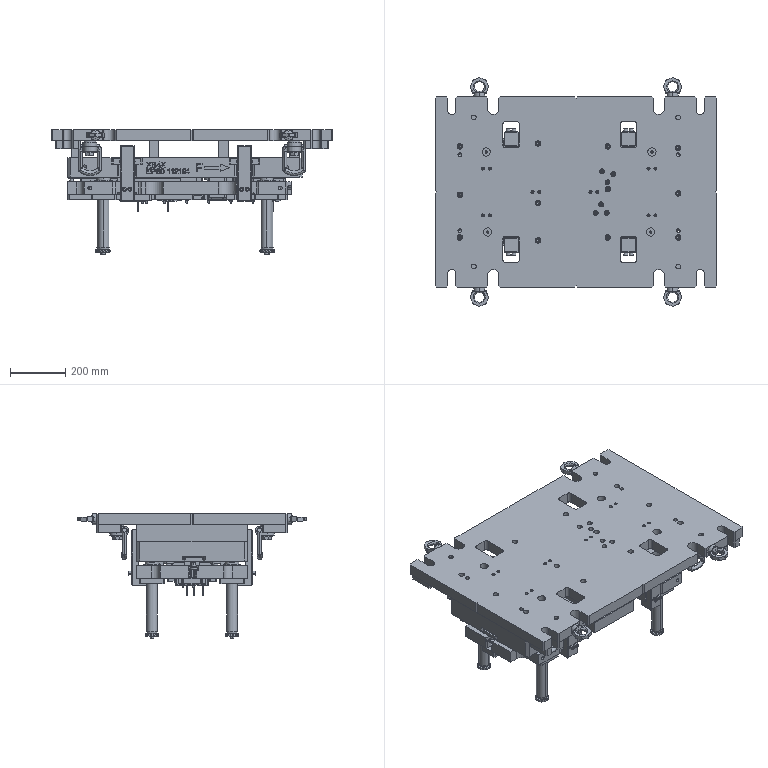Part | CATIA | 217 solids | 11279 faces | volume 70681805 mm3 | plane 6717 | cylinder 2711 | spline 756 | cone 614 | torus 346 | other 82 | sphere 53 | commonest cylinder face diameters 10 x351 11 x194 9 x186 15 x158 20 x150 6.8 x102